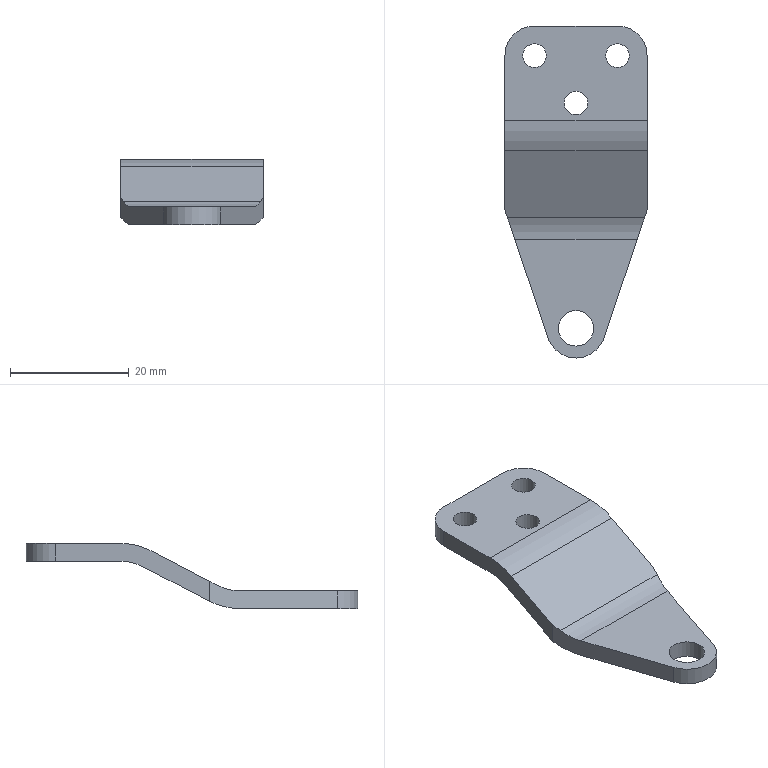Part | STEP file | 1-69.6 | 1 solid | 22 faces | box 24 x 56 x 11 mm | volume 3285 mm3 | plane 11 | cylinder 11 | commonest cylinder face diameters 4 x3 10 x3 16 x2 22 x2 6 x1